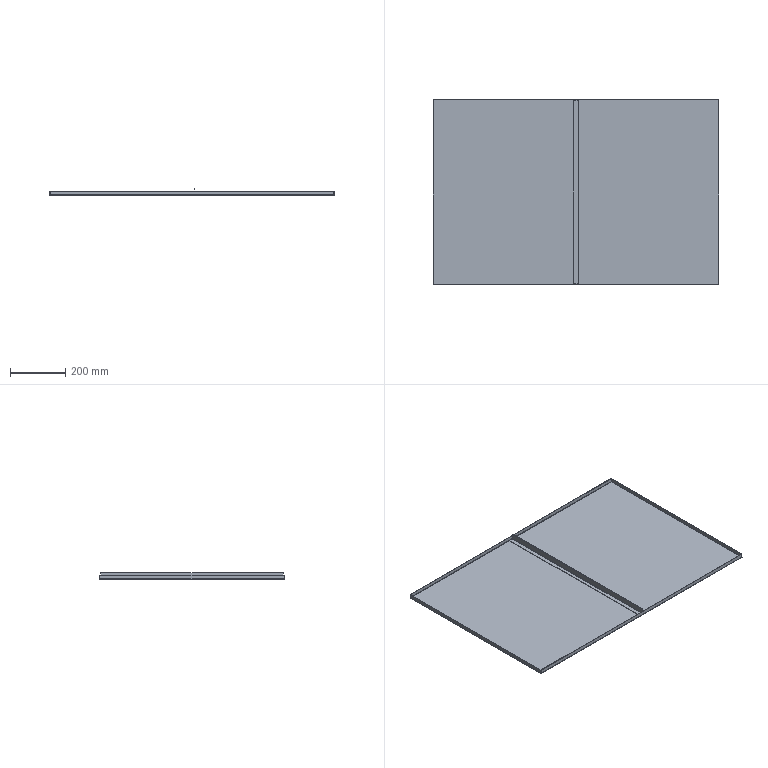Part | SolidWorks | 2 solids | 52 faces | box 1030 x 670.001 x 23 mm | volume 1137543 mm3 | plane 34 | cylinder 10 | spline 8 | commonest cylinder face diameters 0.2 x5 3.2 x5